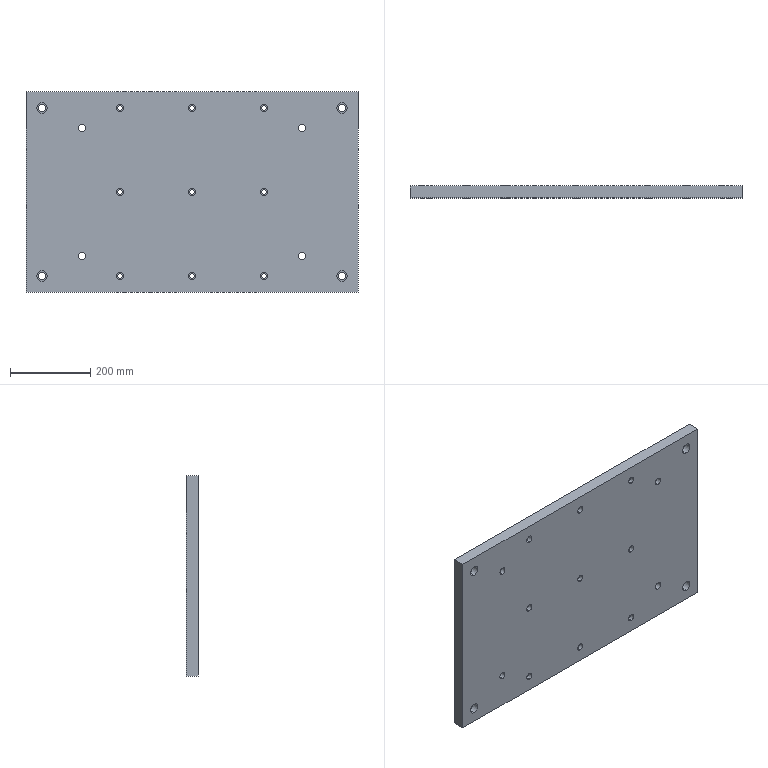Part | STEP file | OP10-014_lower plate (R) | 1 solid | 99 faces | box 830 x 30 x 500 mm | volume 12317635 mm3 | cylinder 68 | plane 23 | cone 8 | commonest cylinder face diameters 18 x34 11 x18 26 x8 30 x8